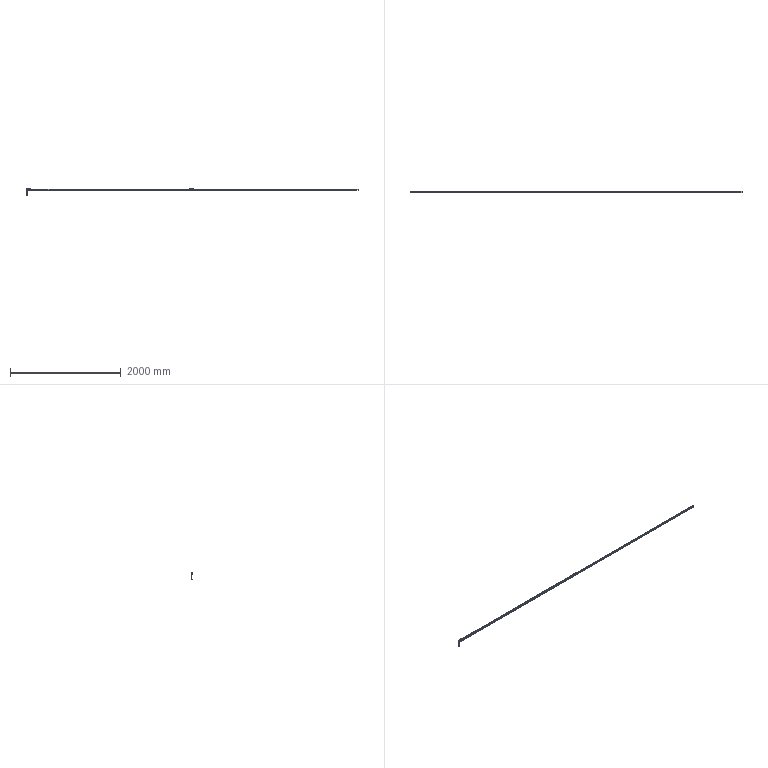Part | STEP file | ASND-0110-Q1_1 | 1 solid | 444 faces | box 5993 x 32 x 129.35 mm | volume 1768651 mm3 | plane 281 | cylinder 135 | cone 26 | other 2 | commonest cylinder face diameters 32 x22 31 x19 24 x18 4.134 x16 12 x12 6 x8